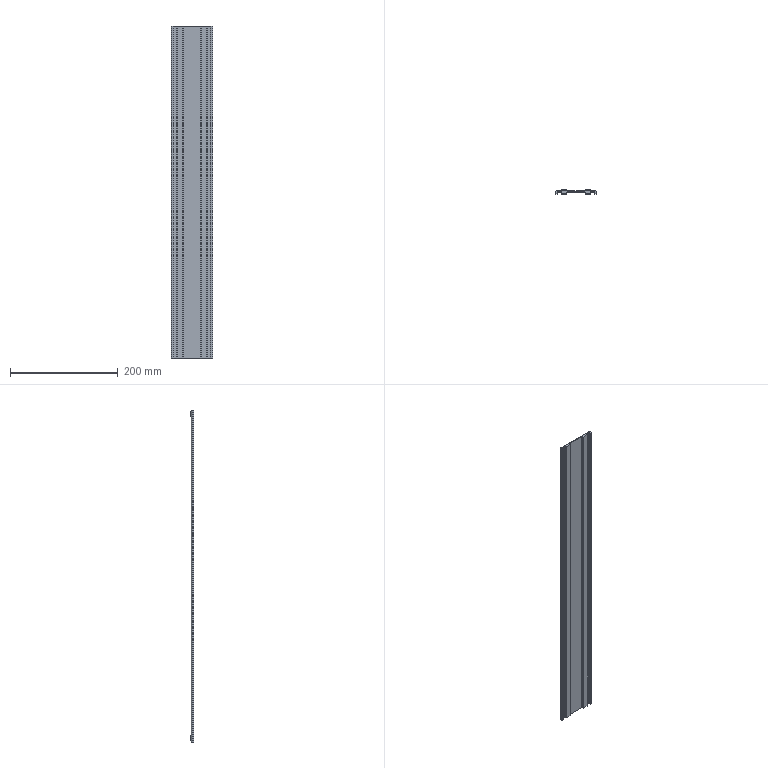Part | STEP file | LX4520CP-MX-B1-590_c | 1 solid | 64 faces | box 77 x 6.5 x 615 mm | volume 143031 mm3 | plane 50 | cylinder 14 | commonest cylinder face diameters 2 x8 9 x4 6 x2